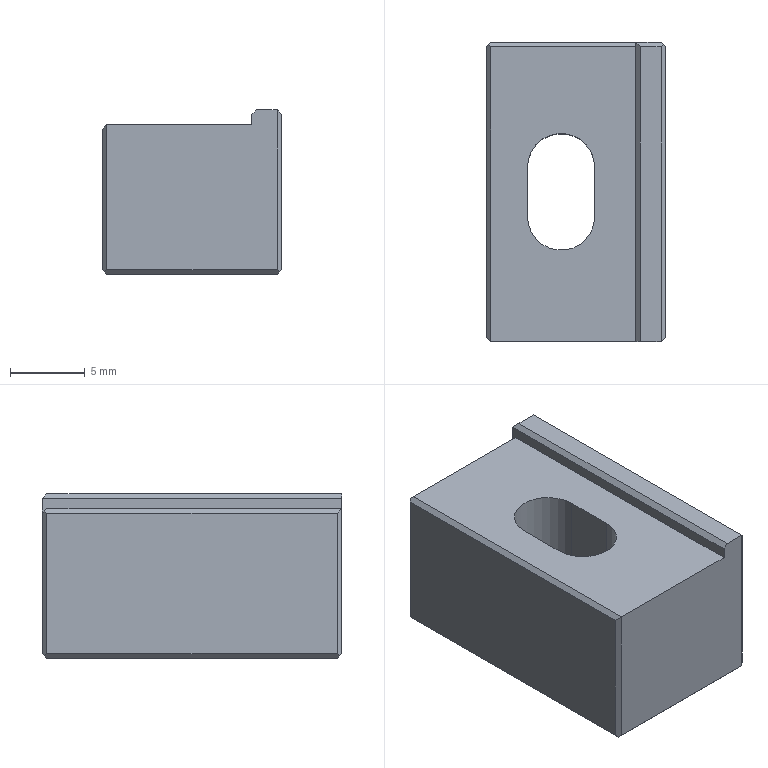Part | NX | 1 solid | 25 faces | box 12 x 20 x 11 mm | volume 2125 mm3 | plane 23 | cylinder 2 | commonest cylinder face diameters 4.5 x2
STEP:
#1=CARTESIAN_POINT('',(2266.8,91.3,-83.));
#2=VERTEX_POINT('',#1);
#3=CARTESIAN_POINT('',(2278.2,91.3,-83.));
#4=VERTEX_POINT('',#3);
#5=CARTESIAN_POINT('',(2272.5,91.3,-83.));
#6=DIRECTION('',(1.,0.,0.));
#7=VECTOR('',#6,1000.);
#8=LINE('',#5,#7);
#9=EDGE_CURVE('',#2,#4,#8,.T.);
#10=ORIENTED_EDGE('',*,*,#9,.F.);
#11=CARTESIAN_POINT('',(2266.8,110.7,-83.));
#12=VERTEX_POINT('',#11);
#13=CARTESIAN_POINT('',(2266.8,101.,-83.));
#14=DIRECTION('',(0.,-1.,0.));
#15=VECTOR('',#14,1000.);
#16=LINE('',#13,#15);
#17=EDGE_CURVE('',#12,#2,#16,.T.);
#18=ORIENTED_EDGE('',*,*,#17,.F.);
#19=CARTESIAN_POINT('',(2278.2,110.7,-83.));
#20=VERTEX_POINT('',#19);
#21=CARTESIAN_POINT('',(2272.5,110.7,-83.));
#22=DIRECTION('',(-1.,0.,0.));
#23=VECTOR('',#22,1000.);
#24=LINE('',#21,#23);
#25=EDGE_CURVE('',#20,#12,#24,.T.);
#26=ORIENTED_EDGE('',*,*,#25,.F.);
#27=CARTESIAN_POINT('',(2278.2,101.,-83.));
#28=DIRECTION('',(0.,-1.,0.));
#29=VECTOR('',#28,1000.);
#30=LINE('',#27,#29);
#31=EDGE_CURVE('',#20,#4,#30,.T.);
#32=ORIENTED_EDGE('',*,*,#31,.T.);
#33=EDGE_LOOP('',(#10,#18,#26,#32));
#34=FACE_BOUND('',#33,.T.);
#35=CARTESIAN_POINT('',(2273.75,99.35,-83.));
#36=VERTEX_POINT('',#35);
#37=CARTESIAN_POINT('',(2269.25,99.35,-83.));
#38=VERTEX_POINT('',#37);
#39=CARTESIAN_POINT('',(2271.5,99.35,-83.));
#40=DIRECTION('',(0.,0.,-1.));
#41=DIRECTION('',(-1.,0.,0.));
#42=AXIS2_PLACEMENT_3D('',#39,#40,#41);
#43=CIRCLE('',#42,2.25);
#44=EDGE_CURVE('',#36,#38,#43,.T.);
#45=ORIENTED_EDGE('',*,*,#44,.F.);
#46=CARTESIAN_POINT('',(2273.75,102.65,-83.));
#47=VERTEX_POINT('',#46);
#48=CARTESIAN_POINT('',(2273.75,45.25,-83.));
#49=DIRECTION('',(0.,1.,0.));
#50=VECTOR('',#49,1000.);
#51=LINE('',#48,#50);
#52=EDGE_CURVE('',#36,#47,#51,.T.);
#53=ORIENTED_EDGE('',*,*,#52,.T.);
#54=CARTESIAN_POINT('',(2269.25,102.65,-83.));
#55=VERTEX_POINT('',#54);
#56=CARTESIAN_POINT('',(2271.5,102.65,-83.));
#57=DIRECTION('',(0.,0.,-1.));
#58=DIRECTION('',(-1.,0.,0.));
#59=AXIS2_PLACEMENT_3D('',#56,#57,#58);
#60=CIRCLE('',#59,2.25);
#61=EDGE_CURVE('',#55,#47,#60,.T.);
#62=ORIENTED_EDGE('',*,*,#61,.F.);
#63=CARTESIAN_POINT('',(2269.25,45.25,-83.));
#64=DIRECTION('',(0.,-1.,0.));
#65=VECTOR('',#64,1000.);
#66=LINE('',#63,#65);
#67=EDGE_CURVE('',#55,#38,#66,.T.);
#68=ORIENTED_EDGE('',*,*,#67,.T.);
#69=EDGE_LOOP('',(#45,#53,#62,#68));
#70=FACE_BOUND('',#69,.T.);
#71=CARTESIAN_POINT('',(2266.5,125.,-83.));
#72=DIRECTION('',(0.,0.,-1.));
#73=DIRECTION('',(0.,-1.,0.));
#74=AXIS2_PLACEMENT_3D('',#71,#72,#73);
#75=PLANE('',#74);
#76=ADVANCED_FACE('',(#34,#70),#75,.T.);
#77=CARTESIAN_POINT('',(2278.2,111.,-72.3));
#78=VERTEX_POINT('',#77);
#79=CARTESIAN_POINT('',(2276.5,111.,-72.3));
#80=VERTEX_POINT('',#79);
#81=CARTESIAN_POINT('',(2277.5,111.,-72.3));
#82=DIRECTION('',(-1.,0.,0.));
#83=VECTOR('',#82,1000.);
#84=LINE('',#81,#83);
#85=EDGE_CURVE('',#78,#80,#84,.T.);
#86=ORIENTED_EDGE('',*,*,#85,.F.);
#87=CARTESIAN_POINT('',(2278.2,111.,-82.7));
#88=VERTEX_POINT('',#87);
#89=CARTESIAN_POINT('',(2278.2,111.,-77.5));
#90=DIRECTION('',(0.,0.,-1.));
#91=VECTOR('',#90,1000.);
#92=LINE('',#89,#91);
#93=EDGE_CURVE('',#78,#88,#92,.T.);
#94=ORIENTED_EDGE('',*,*,#93,.T.);
#95=CARTESIAN_POINT('',(2266.8,111.,-82.7));
#96=VERTEX_POINT('',#95);
#97=CARTESIAN_POINT('',(2272.5,111.,-82.7));
#98=DIRECTION('',(-1.,0.,0.));
#99=VECTOR('',#98,1000.);
#100=LINE('',#97,#99);
#101=EDGE_CURVE('',#88,#96,#100,.T.);
#102=ORIENTED_EDGE('',*,*,#101,.T.);
#103=CARTESIAN_POINT('',(2266.8,111.,-73.3));
#104=VERTEX_POINT('',#103);
#105=CARTESIAN_POINT('',(2266.8,111.,-78.));
#106=DIRECTION('',(0.,0.,-1.));
#107=VECTOR('',#106,1000.);
#108=LINE('',#105,#107);
#109=EDGE_CURVE('',#104,#96,#108,.T.);
#110=ORIENTED_EDGE('',*,*,#109,.F.);
#111=CARTESIAN_POINT('',(2276.5,111.,-73.3));
#112=VERTEX_POINT('',#111);
#113=CARTESIAN_POINT('',(2271.5,111.,-73.3));
#114=DIRECTION('',(-1.,0.,0.));
#115=VECTOR('',#114,1000.);
#116=LINE('',#113,#115);
#117=EDGE_CURVE('',#112,#104,#116,.T.);
#118=ORIENTED_EDGE('',*,*,#117,.F.);
#119=CARTESIAN_POINT('',(2276.5,111.,-12.));
#120=DIRECTION('',(0.,0.,1.));
#121=VECTOR('',#120,1000.);
#122=LINE('',#119,#121);
#123=EDGE_CURVE('',#112,#80,#122,.T.);
#124=ORIENTED_EDGE('',*,*,#123,.T.);
#125=EDGE_LOOP('',(#86,#94,#102,#110,#118,#124));
#126=FACE_BOUND('',#125,.T.);
#127=CARTESIAN_POINT('',(2266.5,111.,-72.));
#128=DIRECTION('',(0.,1.,0.));
#129=DIRECTION('',(1.,0.,0.));
#130=AXIS2_PLACEMENT_3D('',#127,#128,#129);
#131=PLANE('',#130);
#132=ADVANCED_FACE('',(#126),#131,.T.);
#133=CARTESIAN_POINT('',(2276.8,91.,-72.));
#134=VERTEX_POINT('',#133);
#135=CARTESIAN_POINT('',(2276.8,110.7,-72.));
#136=VERTEX_POINT('',#135);
#137=CARTESIAN_POINT('',(2276.8,101.,-72.));
#138=DIRECTION('',(0.,1.,0.));
#139=VECTOR('',#138,1000.);
#140=LINE('',#137,#139);
#141=EDGE_CURVE('',#134,#136,#140,.T.);
#142=ORIENTED_EDGE('',*,*,#141,.F.);
#143=CARTESIAN_POINT('',(2278.2,91.,-72.));
#144=VERTEX_POINT('',#143);
#145=CARTESIAN_POINT('',(2266.5,91.,-72.));
#146=DIRECTION('',(1.,0.,0.));
#147=VECTOR('',#146,1000.);
#148=LINE('',#145,#147);
#149=EDGE_CURVE('',#134,#144,#148,.T.);
#150=ORIENTED_EDGE('',*,*,#149,.T.);
#151=CARTESIAN_POINT('',(2278.2,110.7,-72.));
#152=VERTEX_POINT('',#151);
#153=CARTESIAN_POINT('',(2278.2,101.,-72.));
#154=DIRECTION('',(0.,1.,0.));
#155=VECTOR('',#154,1000.);
#156=LINE('',#153,#155);
#157=EDGE_CURVE('',#144,#152,#156,.T.);
#158=ORIENTED_EDGE('',*,*,#157,.T.);
#159=CARTESIAN_POINT('',(2277.5,110.7,-72.));
#160=DIRECTION('',(-1.,0.,0.));
#161=VECTOR('',#160,1000.);
#162=LINE('',#159,#161);
#163=EDGE_CURVE('',#152,#136,#162,.T.);
#164=ORIENTED_EDGE('',*,*,#163,.T.);
#165=EDGE_LOOP('',(#142,#150,#158,#164));
#166=FACE_BOUND('',#165,.T.);
#167=CARTESIAN_POINT('',(2266.5,91.,-72.));
#168=DIRECTION('',(0.,0.,1.));
#169=DIRECTION('',(1.,0.,0.));
#170=AXIS2_PLACEMENT_3D('',#167,#168,#169);
#171=PLANE('',#170);
#172=ADVANCED_FACE('',(#166),#171,.T.);
#173=CARTESIAN_POINT('',(2276.5,91.,-73.));
#174=VERTEX_POINT('',#173);
#175=CARTESIAN_POINT('',(2276.5,91.,-72.3));
#176=VERTEX_POINT('',#175);
#177=CARTESIAN_POINT('',(2276.5,91.,-12.));
#178=DIRECTION('',(0.,0.,1.));
#179=VECTOR('',#178,1000.);
#180=LINE('',#177,#179);
#181=EDGE_CURVE('',#174,#176,#180,.T.);
#182=ORIENTED_EDGE('',*,*,#181,.F.);
#183=CARTESIAN_POINT('',(2266.8,91.,-73.));
#184=VERTEX_POINT('',#183);
#185=CARTESIAN_POINT('',(2266.5,91.,-73.));
#186=DIRECTION('',(-1.,0.,0.));
#187=VECTOR('',#186,1000.);
#188=LINE('',#185,#187);
#189=EDGE_CURVE('',#174,#184,#188,.T.);
#190=ORIENTED_EDGE('',*,*,#189,.T.);
#191=CARTESIAN_POINT('',(2266.8,91.,-82.7));
#192=VERTEX_POINT('',#191);
#193=CARTESIAN_POINT('',(2266.8,91.,-78.));
#194=DIRECTION('',(0.,0.,1.));
#195=VECTOR('',#194,1000.);
#196=LINE('',#193,#195);
#197=EDGE_CURVE('',#192,#184,#196,.T.);
#198=ORIENTED_EDGE('',*,*,#197,.F.);
#199=CARTESIAN_POINT('',(2278.2,91.,-82.7));
#200=VERTEX_POINT('',#199);
#201=CARTESIAN_POINT('',(2272.5,91.,-82.7));
#202=DIRECTION('',(1.,0.,0.));
#203=VECTOR('',#202,1000.);
#204=LINE('',#201,#203);
#205=EDGE_CURVE('',#192,#200,#204,.T.);
#206=ORIENTED_EDGE('',*,*,#205,.T.);
#207=CARTESIAN_POINT('',(2278.2,91.,-77.5));
#208=DIRECTION('',(0.,0.,1.));
#209=VECTOR('',#208,1000.);
#210=LINE('',#207,#209);
#211=EDGE_CURVE('',#200,#144,#210,.T.);
#212=ORIENTED_EDGE('',*,*,#211,.T.);
#213=ORIENTED_EDGE('',*,*,#149,.F.);
#214=CARTESIAN_POINT('',(2266.5,91.,-82.3));
#215=DIRECTION('',(-0.7071,0.,-0.7071));
#216=VECTOR('',#215,1000.);
#217=LINE('',#214,#216);
#218=EDGE_CURVE('',#134,#176,#217,.T.);
#219=ORIENTED_EDGE('',*,*,#218,.T.);
#220=EDGE_LOOP('',(#182,#190,#198,#206,#212,#213,#219));
#221=FACE_BOUND('',#220,.T.);
#222=CARTESIAN_POINT('',(2266.5,91.,-81.));
#223=DIRECTION('',(0.,-1.,0.));
#224=DIRECTION('',(0.,0.,-1.));
#225=AXIS2_PLACEMENT_3D('',#222,#223,#224);
#226=PLANE('',#225);
#227=ADVANCED_FACE('',(#221),#226,.T.);
#228=CARTESIAN_POINT('',(2266.8,110.7,-73.));
#229=VERTEX_POINT('',#228);
#230=CARTESIAN_POINT('',(2266.8,101.,-73.));
#231=DIRECTION('',(0.,1.,0.));
#232=VECTOR('',#231,1000.);
#233=LINE('',#230,#232);
#234=EDGE_CURVE('',#184,#229,#233,.T.);
#235=ORIENTED_EDGE('',*,*,#234,.F.);
#236=ORIENTED_EDGE('',*,*,#189,.F.);
#237=CARTESIAN_POINT('',(2276.5,110.7,-73.));
#238=VERTEX_POINT('',#237);
#239=CARTESIAN_POINT('',(2276.5,45.25,-73.));
#240=DIRECTION('',(0.,-1.,0.));
#241=VECTOR('',#240,1000.);
#242=LINE('',#239,#241);
#243=EDGE_CURVE('',#238,#174,#242,.T.);
#244=ORIENTED_EDGE('',*,*,#243,.F.);
#245=CARTESIAN_POINT('',(2271.5,110.7,-73.));
#246=DIRECTION('',(-1.,0.,0.));
#247=VECTOR('',#246,1000.);
#248=LINE('',#245,#247);
#249=EDGE_CURVE('',#238,#229,#248,.T.);
#250=ORIENTED_EDGE('',*,*,#249,.T.);
#251=EDGE_LOOP('',(#235,#236,#244,#250));
#252=FACE_BOUND('',#251,.T.);
#253=CARTESIAN_POINT('',(2273.75,99.35,-73.));
#254=VERTEX_POINT('',#253);
#255=CARTESIAN_POINT('',(2269.25,99.35,-73.));
#256=VERTEX_POINT('',#255);
#257=CARTESIAN_POINT('',(2271.5,99.35,-73.));
#258=DIRECTION('',(0.,0.,-1.));
#259=DIRECTION('',(-1.,0.,0.));
#260=AXIS2_PLACEMENT_3D('',#257,#258,#259);
#261=CIRCLE('',#260,2.25);
#262=EDGE_CURVE('',#254,#256,#261,.T.);
#263=ORIENTED_EDGE('',*,*,#262,.T.);
#264=CARTESIAN_POINT('',(2269.25,102.65,-73.));
#265=VERTEX_POINT('',#264);
#266=CARTESIAN_POINT('',(2269.25,45.25,-73.));
#267=DIRECTION('',(0.,1.,0.));
#268=VECTOR('',#267,1000.);
#269=LINE('',#266,#268);
#270=EDGE_CURVE('',#256,#265,#269,.T.);
#271=ORIENTED_EDGE('',*,*,#270,.T.);
#272=CARTESIAN_POINT('',(2273.75,102.65,-73.));
#273=VERTEX_POINT('',#272);
#274=CARTESIAN_POINT('',(2271.5,102.65,-73.));
#275=DIRECTION('',(0.,0.,-1.));
#276=DIRECTION('',(-1.,0.,0.));
#277=AXIS2_PLACEMENT_3D('',#274,#275,#276);
#278=CIRCLE('',#277,2.25);
#279=EDGE_CURVE('',#265,#273,#278,.T.);
#280=ORIENTED_EDGE('',*,*,#279,.T.);
#281=CARTESIAN_POINT('',(2273.75,45.25,-73.));
#282=DIRECTION('',(0.,-1.,0.));
#283=VECTOR('',#282,1000.);
#284=LINE('',#281,#283);
#285=EDGE_CURVE('',#273,#254,#284,.T.);
#286=ORIENTED_EDGE('',*,*,#285,.T.);
#287=EDGE_LOOP('',(#263,#271,#280,#286));
#288=FACE_BOUND('',#287,.T.);
#289=CARTESIAN_POINT('',(2275.402,98.391,-73.));
#290=DIRECTION('',(0.,0.,1.));
#291=DIRECTION('',(1.,0.,0.));
#292=AXIS2_PLACEMENT_3D('',#289,#290,#291);
#293=PLANE('',#292);
#294=ADVANCED_FACE('',(#252,#288),#293,.T.);
#295=ORIENTED_EDGE('',*,*,#123,.F.);
#296=CARTESIAN_POINT('',(2276.5,49.7,-12.));
#297=DIRECTION('',(0.,0.7071,-0.7071));
#298=VECTOR('',#297,1000.);
#299=LINE('',#296,#298);
#300=EDGE_CURVE('',#238,#112,#299,.T.);
#301=ORIENTED_EDGE('',*,*,#300,.F.);
#302=ORIENTED_EDGE('',*,*,#243,.T.);
#303=ORIENTED_EDGE('',*,*,#181,.T.);
#304=CARTESIAN_POINT('',(2276.5,101.,-72.3));
#305=DIRECTION('',(0.,1.,0.));
#306=VECTOR('',#305,1000.);
#307=LINE('',#304,#306);
#308=EDGE_CURVE('',#176,#80,#307,.T.);
#309=ORIENTED_EDGE('',*,*,#308,.T.);
#310=EDGE_LOOP('',(#295,#301,#302,#303,#309));
#311=FACE_BOUND('',#310,.T.);
#312=CARTESIAN_POINT('',(2276.5,91.,-72.));
#313=DIRECTION('',(1.,0.,0.));
#314=DIRECTION('',(0.,1.,0.));
#315=AXIS2_PLACEMENT_3D('',#312,#313,#314);
#316=PLANE('',#315);
#317=ADVANCED_FACE('',(#311),#316,.F.);
#318=ORIENTED_EDGE('',*,*,#262,.F.);
#319=CARTESIAN_POINT('',(2273.75,99.35,-71.1));
#320=DIRECTION('',(0.,0.,-1.));
#321=VECTOR('',#320,1000.);
#322=LINE('',#319,#321);
#323=EDGE_CURVE('',#254,#36,#322,.T.);
#324=ORIENTED_EDGE('',*,*,#323,.T.);
#325=ORIENTED_EDGE('',*,*,#44,.T.);
#326=CARTESIAN_POINT('',(2269.25,99.35,-71.1));
#327=DIRECTION('',(0.,0.,-1.));
#328=VECTOR('',#327,1000.);
#329=LINE('',#326,#328);
#330=EDGE_CURVE('',#256,#38,#329,.T.);
#331=ORIENTED_EDGE('',*,*,#330,.F.);
#332=EDGE_LOOP('',(#318,#324,#325,#331));
#333=FACE_BOUND('',#332,.T.);
#334=CARTESIAN_POINT('',(2271.5,99.35,-71.1));
#335=DIRECTION('',(0.,0.,-1.));
#336=DIRECTION('',(-1.,0.,0.));
#337=AXIS2_PLACEMENT_3D('',#334,#335,#336);
#338=CYLINDRICAL_SURFACE('',#337,2.25);
#339=ADVANCED_FACE('',(#333),#338,.F.);
#340=ORIENTED_EDGE('',*,*,#285,.F.);
#341=CARTESIAN_POINT('',(2273.75,102.65,-71.1));
#342=DIRECTION('',(0.,0.,-1.));
#343=VECTOR('',#342,1000.);
#344=LINE('',#341,#343);
#345=EDGE_CURVE('',#273,#47,#344,.T.);
#346=ORIENTED_EDGE('',*,*,#345,.T.);
#347=ORIENTED_EDGE('',*,*,#52,.F.);
#348=ORIENTED_EDGE('',*,*,#323,.F.);
#349=EDGE_LOOP('',(#340,#346,#347,#348));
#350=FACE_BOUND('',#349,.T.);
#351=CARTESIAN_POINT('',(2273.75,99.35,-71.1));
#352=DIRECTION('',(1.,0.,0.));
#353=DIRECTION('',(0.,1.,0.));
#354=AXIS2_PLACEMENT_3D('',#351,#352,#353);
#355=PLANE('',#354);
#356=ADVANCED_FACE('',(#350),#355,.F.);
#357=ORIENTED_EDGE('',*,*,#279,.F.);
#358=CARTESIAN_POINT('',(2269.25,102.65,-71.1));
#359=DIRECTION('',(0.,0.,-1.));
#360=VECTOR('',#359,1000.);
#361=LINE('',#358,#360);
#362=EDGE_CURVE('',#265,#55,#361,.T.);
#363=ORIENTED_EDGE('',*,*,#362,.T.);
#364=ORIENTED_EDGE('',*,*,#61,.T.);
#365=ORIENTED_EDGE('',*,*,#345,.F.);
#366=EDGE_LOOP('',(#357,#363,#364,#365));
#367=FACE_BOUND('',#366,.T.);
#368=CARTESIAN_POINT('',(2271.5,102.65,-71.1));
#369=DIRECTION('',(0.,0.,-1.));
#370=DIRECTION('',(-1.,0.,0.));
#371=AXIS2_PLACEMENT_3D('',#368,#369,#370);
#372=CYLINDRICAL_SURFACE('',#371,2.25);
#373=ADVANCED_FACE('',(#367),#372,.F.);
#374=ORIENTED_EDGE('',*,*,#270,.F.);
#375=ORIENTED_EDGE('',*,*,#330,.T.);
#376=ORIENTED_EDGE('',*,*,#67,.F.);
#377=ORIENTED_EDGE('',*,*,#362,.F.);
#378=EDGE_LOOP('',(#374,#375,#376,#377));
#379=FACE_BOUND('',#378,.T.);
#380=CARTESIAN_POINT('',(2269.25,102.65,-71.1));
#381=DIRECTION('',(-1.,0.,0.));
#382=DIRECTION('',(0.,0.,1.));
#383=AXIS2_PLACEMENT_3D('',#380,#381,#382);
#384=PLANE('',#383);
#385=ADVANCED_FACE('',(#379),#384,.F.);
#386=ORIENTED_EDGE('',*,*,#25,.T.);
#387=CARTESIAN_POINT('',(2266.65,110.85,-82.85));
#388=VERTEX_POINT('',#387);
#389=CARTESIAN_POINT('',(2266.5,111.,-82.7));
#390=DIRECTION('',(0.5774,-0.5774,-0.5774));
#391=VECTOR('',#390,1000.);
#392=LINE('',#389,#391);
#393=EDGE_CURVE('',#388,#12,#392,.T.);
#394=ORIENTED_EDGE('',*,*,#393,.F.);
#395=CARTESIAN_POINT('',(2266.5,110.7,-83.));
#396=DIRECTION('',(-0.5774,-0.5774,-0.5774));
#397=VECTOR('',#396,1000.);
#398=LINE('',#395,#397);
#399=EDGE_CURVE('',#96,#388,#398,.T.);
#400=ORIENTED_EDGE('',*,*,#399,.F.);
#401=ORIENTED_EDGE('',*,*,#101,.F.);
#402=CARTESIAN_POINT('',(2278.35,110.85,-82.85));
#403=VERTEX_POINT('',#402);
#404=CARTESIAN_POINT('',(2266.5,122.7,-71.));
#405=DIRECTION('',(0.5774,-0.5774,-0.5774));
#406=VECTOR('',#405,1000.);
#407=LINE('',#404,#406);
#408=EDGE_CURVE('',#88,#403,#407,.T.);
#409=ORIENTED_EDGE('',*,*,#408,.T.);
#410=CARTESIAN_POINT('',(2266.5,99.,-94.7));
#411=DIRECTION('',(-0.5774,-0.5774,-0.5774));
#412=VECTOR('',#411,1000.);
#413=LINE('',#410,#412);
#414=EDGE_CURVE('',#403,#20,#413,.T.);
#415=ORIENTED_EDGE('',*,*,#414,.T.);
#416=EDGE_LOOP('',(#386,#394,#400,#401,#409,#415));
#417=FACE_BOUND('',#416,.T.);
#418=CARTESIAN_POINT('',(2272.5,110.85,-82.85));
#419=DIRECTION('',(0.,-0.7071,0.7071));
#420=DIRECTION('',(-1.,0.,0.));
#421=AXIS2_PLACEMENT_3D('',#418,#419,#420);
#422=PLANE('',#421);
#423=ADVANCED_FACE('',(#417),#422,.F.);
#424=ORIENTED_EDGE('',*,*,#249,.F.);
#425=ORIENTED_EDGE('',*,*,#300,.T.);
#426=ORIENTED_EDGE('',*,*,#117,.T.);
#427=CARTESIAN_POINT('',(2266.65,110.85,-73.15));
#428=VERTEX_POINT('',#427);
#429=CARTESIAN_POINT('',(2266.5,110.7,-73.));
#430=DIRECTION('',(0.5774,0.5774,-0.5774));
#431=VECTOR('',#430,1000.);
#432=LINE('',#429,#431);
#433=EDGE_CURVE('',#428,#104,#432,.T.);
#434=ORIENTED_EDGE('',*,*,#433,.F.);
#435=CARTESIAN_POINT('',(2266.5,111.,-73.3));
#436=DIRECTION('',(-0.5774,0.5774,-0.5774));
#437=VECTOR('',#436,1000.);
#438=LINE('',#435,#437);
#439=EDGE_CURVE('',#229,#428,#438,.T.);
#440=ORIENTED_EDGE('',*,*,#439,.F.);
#441=EDGE_LOOP('',(#424,#425,#426,#434,#440));
#442=FACE_BOUND('',#441,.T.);
#443=CARTESIAN_POINT('',(2271.5,110.85,-73.15));
#444=DIRECTION('',(0.,0.7071,0.7071));
#445=DIRECTION('',(1.,0.,0.));
#446=AXIS2_PLACEMENT_3D('',#443,#444,#445);
#447=PLANE('',#446);
#448=ADVANCED_FACE('',(#442),#447,.T.);
#449=ORIENTED_EDGE('',*,*,#85,.T.);
#450=CARTESIAN_POINT('',(2266.5,121.,-82.3));
#451=DIRECTION('',(0.5774,-0.5774,0.5774));
#452=VECTOR('',#451,1000.);
#453=LINE('',#450,#452);
#454=EDGE_CURVE('',#80,#136,#453,.T.);
#455=ORIENTED_EDGE('',*,*,#454,.T.);
#456=ORIENTED_EDGE('',*,*,#163,.F.);
#457=CARTESIAN_POINT('',(2278.35,110.85,-72.15));
#458=VERTEX_POINT('',#457);
#459=CARTESIAN_POINT('',(2266.5,99.,-60.3));
#460=DIRECTION('',(0.5774,0.5774,-0.5774));
#461=VECTOR('',#460,1000.);
#462=LINE('',#459,#461);
#463=EDGE_CURVE('',#152,#458,#462,.T.);
#464=ORIENTED_EDGE('',*,*,#463,.T.);
#465=CARTESIAN_POINT('',(2266.5,122.7,-84.));
#466=DIRECTION('',(-0.5774,0.5774,-0.5774));
#467=VECTOR('',#466,1000.);
#468=LINE('',#465,#467);
#469=EDGE_CURVE('',#458,#78,#468,.T.);
#470=ORIENTED_EDGE('',*,*,#469,.T.);
#471=EDGE_LOOP('',(#449,#455,#456,#464,#470));
#472=FACE_BOUND('',#471,.T.);
#473=CARTESIAN_POINT('',(2277.5,110.85,-72.15));
#474=DIRECTION('',(0.,-0.7071,-0.7071));
#475=DIRECTION('',(0.,-0.7071,0.7071));
#476=AXIS2_PLACEMENT_3D('',#473,#474,#475);
#477=PLANE('',#476);
#478=ADVANCED_FACE('',(#472),#477,.F.);
#479=ORIENTED_EDGE('',*,*,#141,.T.);
#480=ORIENTED_EDGE('',*,*,#454,.F.);
#481=ORIENTED_EDGE('',*,*,#308,.F.);
#482=ORIENTED_EDGE('',*,*,#218,.F.);
#483=EDGE_LOOP('',(#479,#480,#481,#482));
#484=FACE_BOUND('',#483,.T.);
#485=CARTESIAN_POINT('',(2276.65,101.,-72.15));
#486=DIRECTION('',(0.7071,0.,-0.7071));
#487=DIRECTION('',(0.,-1.,0.));
#488=AXIS2_PLACEMENT_3D('',#485,#486,#487);
#489=PLANE('',#488);
#490=ADVANCED_FACE('',(#484),#489,.F.);
#491=ORIENTED_EDGE('',*,*,#234,.T.);
#492=ORIENTED_EDGE('',*,*,#439,.T.);
#493=CARTESIAN_POINT('',(2266.5,110.7,-73.3));
#494=VERTEX_POINT('',#493);
#495=CARTESIAN_POINT('',(2266.5,110.7,-73.3));
#496=DIRECTION('',(-0.5774,-0.5774,-0.5774));
#497=VECTOR('',#496,1000.);
#498=LINE('',#495,#497);
#499=EDGE_CURVE('',#428,#494,#498,.T.);
#500=ORIENTED_EDGE('',*,*,#499,.T.);
#501=CARTESIAN_POINT('',(2266.5,91.3,-73.3));
#502=VERTEX_POINT('',#501);
#503=CARTESIAN_POINT('',(2266.5,101.,-73.3));
#504=DIRECTION('',(0.,1.,0.));
#505=VECTOR('',#504,1000.);
#506=LINE('',#503,#505);
#507=EDGE_CURVE('',#502,#494,#506,.T.);
#508=ORIENTED_EDGE('',*,*,#507,.F.);
#509=CARTESIAN_POINT('',(2266.5,91.3,-73.3));
#510=DIRECTION('',(-0.5774,0.5774,-0.5774));
#511=VECTOR('',#510,1000.);
#512=LINE('',#509,#511);
#513=EDGE_CURVE('',#184,#502,#512,.T.);
#514=ORIENTED_EDGE('',*,*,#513,.F.);
#515=EDGE_LOOP('',(#491,#492,#500,#508,#514));
#516=FACE_BOUND('',#515,.T.);
#517=CARTESIAN_POINT('',(2266.65,101.,-73.15));
#518=DIRECTION('',(0.7071,0.,-0.7071));
#519=DIRECTION('',(0.,-1.,0.));
#520=AXIS2_PLACEMENT_3D('',#517,#518,#519);
#521=PLANE('',#520);
#522=ADVANCED_FACE('',(#516),#521,.F.);
#523=ORIENTED_EDGE('',*,*,#9,.T.);
#524=CARTESIAN_POINT('',(2278.35,91.15,-82.85));
#525=VERTEX_POINT('',#524);
#526=CARTESIAN_POINT('',(2266.5,103.,-94.7));
#527=DIRECTION('',(0.5774,-0.5774,0.5774));
#528=VECTOR('',#527,1000.);
#529=LINE('',#526,#528);
#530=EDGE_CURVE('',#4,#525,#529,.T.);
#531=ORIENTED_EDGE('',*,*,#530,.T.);
#532=CARTESIAN_POINT('',(2266.5,79.3,-71.));
#533=DIRECTION('',(0.5774,0.5774,-0.5774));
#534=VECTOR('',#533,1000.);
#535=LINE('',#532,#534);
#536=EDGE_CURVE('',#200,#525,#535,.T.);
#537=ORIENTED_EDGE('',*,*,#536,.F.);
#538=ORIENTED_EDGE('',*,*,#205,.F.);
#539=CARTESIAN_POINT('',(2266.65,91.15,-82.85));
#540=VERTEX_POINT('',#539);
#541=CARTESIAN_POINT('',(2266.5,91.3,-83.));
#542=DIRECTION('',(-0.5774,0.5774,-0.5774));
#543=VECTOR('',#542,1000.);
#544=LINE('',#541,#543);
#545=EDGE_CURVE('',#192,#540,#544,.T.);
#546=ORIENTED_EDGE('',*,*,#545,.T.);
#547=CARTESIAN_POINT('',(2266.5,91.,-82.7));
#548=DIRECTION('',(0.5774,0.5774,-0.5774));
#549=VECTOR('',#548,1000.);
#550=LINE('',#547,#549);
#551=EDGE_CURVE('',#540,#2,#550,.T.);
#552=ORIENTED_EDGE('',*,*,#551,.T.);
#553=EDGE_LOOP('',(#523,#531,#537,#538,#546,#552));
#554=FACE_BOUND('',#553,.T.);
#555=CARTESIAN_POINT('',(2272.5,91.15,-82.85));
#556=DIRECTION('',(0.,0.7071,0.7071));
#557=DIRECTION('',(1.,0.,0.));
#558=AXIS2_PLACEMENT_3D('',#555,#556,#557);
#559=PLANE('',#558);
#560=ADVANCED_FACE('',(#554),#559,.F.);
#561=CARTESIAN_POINT('',(2278.5,110.7,-82.7));
#562=VERTEX_POINT('',#561);
#563=CARTESIAN_POINT('',(2278.5,91.3,-82.7));
#564=VERTEX_POINT('',#563);
#565=CARTESIAN_POINT('',(2278.5,101.,-82.7));
#566=DIRECTION('',(0.,-1.,0.));
#567=VECTOR('',#566,1000.);
#568=LINE('',#565,#567);
#569=EDGE_CURVE('',#562,#564,#568,.T.);
#570=ORIENTED_EDGE('',*,*,#569,.F.);
#571=CARTESIAN_POINT('',(2278.5,110.7,-72.3));
#572=VERTEX_POINT('',#571);
#573=CARTESIAN_POINT('',(2278.5,110.7,-77.5));
#574=DIRECTION('',(0.,0.,-1.));
#575=VECTOR('',#574,1000.);
#576=LINE('',#573,#575);
#577=EDGE_CURVE('',#572,#562,#576,.T.);
#578=ORIENTED_EDGE('',*,*,#577,.F.);
#579=CARTESIAN_POINT('',(2278.5,91.3,-72.3));
#580=VERTEX_POINT('',#579);
#581=CARTESIAN_POINT('',(2278.5,101.,-72.3));
#582=DIRECTION('',(0.,1.,0.));
#583=VECTOR('',#582,1000.);
#584=LINE('',#581,#583);
#585=EDGE_CURVE('',#580,#572,#584,.T.);
#586=ORIENTED_EDGE('',*,*,#585,.F.);
#587=CARTESIAN_POINT('',(2278.5,91.3,-77.5));
#588=DIRECTION('',(0.,0.,1.));
#589=VECTOR('',#588,1000.);
#590=LINE('',#587,#589);
#591=EDGE_CURVE('',#564,#580,#590,.T.);
#592=ORIENTED_EDGE('',*,*,#591,.F.);
#593=EDGE_LOOP('',(#570,#578,#586,#592));
#594=FACE_BOUND('',#593,.T.);
#595=CARTESIAN_POINT('',(2278.5,45.25,-12.));
#596=DIRECTION('',(-1.,0.,0.));
#597=DIRECTION('',(0.,0.,1.));
#598=AXIS2_PLACEMENT_3D('',#595,#596,#597);
#599=PLANE('',#598);
#600=ADVANCED_FACE('',(#594),#599,.F.);
#601=ORIENTED_EDGE('',*,*,#577,.T.);
#602=CARTESIAN_POINT('',(2266.5,122.7,-94.7));
#603=DIRECTION('',(-0.5774,0.5774,-0.5774));
#604=VECTOR('',#603,1000.);
#605=LINE('',#602,#604);
#606=EDGE_CURVE('',#562,#403,#605,.T.);
#607=ORIENTED_EDGE('',*,*,#606,.T.);
#608=ORIENTED_EDGE('',*,*,#408,.F.);
#609=ORIENTED_EDGE('',*,*,#93,.F.);
#610=ORIENTED_EDGE('',*,*,#469,.F.);
#611=CARTESIAN_POINT('',(2266.5,122.7,-60.3));
#612=DIRECTION('',(0.5774,-0.5774,-0.5774));
#613=VECTOR('',#612,1000.);
#614=LINE('',#611,#613);
#615=EDGE_CURVE('',#458,#572,#614,.T.);
#616=ORIENTED_EDGE('',*,*,#615,.T.);
#617=EDGE_LOOP('',(#601,#607,#608,#609,#610,#616));
#618=FACE_BOUND('',#617,.T.);
#619=CARTESIAN_POINT('',(2278.35,110.85,-77.5));
#620=DIRECTION('',(-0.7071,-0.7071,0.));
#621=DIRECTION('',(-0.7071,0.7071,0.));
#622=AXIS2_PLACEMENT_3D('',#619,#620,#621);
#623=PLANE('',#622);
#624=ADVANCED_FACE('',(#618),#623,.F.);
#625=ORIENTED_EDGE('',*,*,#591,.T.);
#626=CARTESIAN_POINT('',(2266.5,79.3,-60.3));
#627=DIRECTION('',(-0.5774,-0.5774,0.5774));
#628=VECTOR('',#627,1000.);
#629=LINE('',#626,#628);
#630=EDGE_CURVE('',#580,#144,#629,.T.);
#631=ORIENTED_EDGE('',*,*,#630,.T.);
#632=ORIENTED_EDGE('',*,*,#211,.F.);
#633=ORIENTED_EDGE('',*,*,#536,.T.);
#634=CARTESIAN_POINT('',(2266.5,79.3,-94.7));
#635=DIRECTION('',(0.5774,0.5774,0.5774));
#636=VECTOR('',#635,1000.);
#637=LINE('',#634,#636);
#638=EDGE_CURVE('',#525,#564,#637,.T.);
#639=ORIENTED_EDGE('',*,*,#638,.T.);
#640=EDGE_LOOP('',(#625,#631,#632,#633,#639));
#641=FACE_BOUND('',#640,.T.);
#642=CARTESIAN_POINT('',(2278.35,91.15,-77.5));
#643=DIRECTION('',(-0.7071,0.7071,0.));
#644=DIRECTION('',(0.,0.,1.));
#645=AXIS2_PLACEMENT_3D('',#642,#643,#644);
#646=PLANE('',#645);
#647=ADVANCED_FACE('',(#641),#646,.F.);
#648=ORIENTED_EDGE('',*,*,#585,.T.);
#649=ORIENTED_EDGE('',*,*,#615,.F.);
#650=ORIENTED_EDGE('',*,*,#463,.F.);
#651=ORIENTED_EDGE('',*,*,#157,.F.);
#652=ORIENTED_EDGE('',*,*,#630,.F.);
#653=EDGE_LOOP('',(#648,#649,#650,#651,#652));
#654=FACE_BOUND('',#653,.T.);
#655=CARTESIAN_POINT('',(2278.35,101.,-72.15));
#656=DIRECTION('',(-0.7071,0.,-0.7071));
#657=DIRECTION('',(-0.7071,0.,0.7071));
#658=AXIS2_PLACEMENT_3D('',#655,#656,#657);
#659=PLANE('',#658);
#660=ADVANCED_FACE('',(#654),#659,.F.);
#661=ORIENTED_EDGE('',*,*,#569,.T.);
#662=ORIENTED_EDGE('',*,*,#638,.F.);
#663=ORIENTED_EDGE('',*,*,#530,.F.);
#664=ORIENTED_EDGE('',*,*,#31,.F.);
#665=ORIENTED_EDGE('',*,*,#414,.F.);
#666=ORIENTED_EDGE('',*,*,#606,.F.);
#667=EDGE_LOOP('',(#661,#662,#663,#664,#665,#666));
#668=FACE_BOUND('',#667,.T.);
#669=CARTESIAN_POINT('',(2278.35,101.,-82.85));
#670=DIRECTION('',(-0.7071,0.,0.7071));
#671=DIRECTION('',(0.,1.,0.));
#672=AXIS2_PLACEMENT_3D('',#669,#670,#671);
#673=PLANE('',#672);
#674=ADVANCED_FACE('',(#668),#673,.F.);
#675=CARTESIAN_POINT('',(2266.5,91.3,-82.7));
#676=VERTEX_POINT('',#675);
#677=CARTESIAN_POINT('',(2266.5,91.3,-78.));
#678=DIRECTION('',(0.,0.,1.));
#679=VECTOR('',#678,1000.);
#680=LINE('',#677,#679);
#681=EDGE_CURVE('',#676,#502,#680,.T.);
#682=ORIENTED_EDGE('',*,*,#681,.T.);
#683=ORIENTED_EDGE('',*,*,#507,.T.);
#684=CARTESIAN_POINT('',(2266.5,110.7,-82.7));
#685=VERTEX_POINT('',#684);
#686=CARTESIAN_POINT('',(2266.5,110.7,-78.));
#687=DIRECTION('',(0.,0.,-1.));
#688=VECTOR('',#687,1000.);
#689=LINE('',#686,#688);
#690=EDGE_CURVE('',#494,#685,#689,.T.);
#691=ORIENTED_EDGE('',*,*,#690,.T.);
#692=CARTESIAN_POINT('',(2266.5,101.,-82.7));
#693=DIRECTION('',(0.,-1.,0.));
#694=VECTOR('',#693,1000.);
#695=LINE('',#692,#694);
#696=EDGE_CURVE('',#685,#676,#695,.T.);
#697=ORIENTED_EDGE('',*,*,#696,.T.);
#698=EDGE_LOOP('',(#682,#683,#691,#697));
#699=FACE_BOUND('',#698,.T.);
#700=CARTESIAN_POINT('',(2266.5,45.25,-12.));
#701=DIRECTION('',(-1.,0.,0.));
#702=DIRECTION('',(0.,0.,1.));
#703=AXIS2_PLACEMENT_3D('',#700,#701,#702);
#704=PLANE('',#703);
#705=ADVANCED_FACE('',(#699),#704,.T.);
#706=ORIENTED_EDGE('',*,*,#696,.F.);
#707=CARTESIAN_POINT('',(2266.5,110.7,-82.7));
#708=DIRECTION('',(0.5774,0.5774,-0.5774));
#709=VECTOR('',#708,1000.);
#710=LINE('',#707,#709);
#711=EDGE_CURVE('',#685,#388,#710,.T.);
#712=ORIENTED_EDGE('',*,*,#711,.T.);
#713=ORIENTED_EDGE('',*,*,#393,.T.);
#714=ORIENTED_EDGE('',*,*,#17,.T.);
#715=ORIENTED_EDGE('',*,*,#551,.F.);
#716=CARTESIAN_POINT('',(2266.5,91.3,-82.7));
#717=DIRECTION('',(-0.5774,0.5774,0.5774));
#718=VECTOR('',#717,1000.);
#719=LINE('',#716,#718);
#720=EDGE_CURVE('',#540,#676,#719,.T.);
#721=ORIENTED_EDGE('',*,*,#720,.T.);
#722=EDGE_LOOP('',(#706,#712,#713,#714,#715,#721));
#723=FACE_BOUND('',#722,.T.);
#724=CARTESIAN_POINT('',(2266.65,101.,-82.85));
#725=DIRECTION('',(-0.7071,0.,-0.7071));
#726=DIRECTION('',(-0.7071,0.,0.7071));
#727=AXIS2_PLACEMENT_3D('',#724,#725,#726);
#728=PLANE('',#727);
#729=ADVANCED_FACE('',(#723),#728,.T.);
#730=ORIENTED_EDGE('',*,*,#690,.F.);
#731=ORIENTED_EDGE('',*,*,#499,.F.);
#732=ORIENTED_EDGE('',*,*,#433,.T.);
#733=ORIENTED_EDGE('',*,*,#109,.T.);
#734=ORIENTED_EDGE('',*,*,#399,.T.);
#735=ORIENTED_EDGE('',*,*,#711,.F.);
#736=EDGE_LOOP('',(#730,#731,#732,#733,#734,#735));
#737=FACE_BOUND('',#736,.T.);
#738=CARTESIAN_POINT('',(2266.65,110.85,-78.));
#739=DIRECTION('',(-0.7071,0.7071,0.));
#740=DIRECTION('',(0.,0.,1.));
#741=AXIS2_PLACEMENT_3D('',#738,#739,#740);
#742=PLANE('',#741);
#743=ADVANCED_FACE('',(#737),#742,.T.);
#744=ORIENTED_EDGE('',*,*,#681,.F.);
#745=ORIENTED_EDGE('',*,*,#720,.F.);
#746=ORIENTED_EDGE('',*,*,#545,.F.);
#747=ORIENTED_EDGE('',*,*,#197,.T.);
#748=ORIENTED_EDGE('',*,*,#513,.T.);
#749=EDGE_LOOP('',(#744,#745,#746,#747,#748));
#750=FACE_BOUND('',#749,.T.);
#751=CARTESIAN_POINT('',(2266.65,91.15,-78.));
#752=DIRECTION('',(-0.7071,-0.7071,0.));
#753=DIRECTION('',(-0.7071,0.7071,0.));
#754=AXIS2_PLACEMENT_3D('',#751,#752,#753);
#755=PLANE('',#754);
#756=ADVANCED_FACE('',(#750),#755,.T.);
#757=CLOSED_SHELL('',(#76,#132,#172,#227,#294,#317,#339,#356,#373,#385,#423,#448,#478,#490,#522,#560,#600,#624,#647,#660,#674,#705,#729,#743,#756));
#758=MANIFOLD_SOLID_BREP('',#757);
#759=(LENGTH_UNIT()NAMED_UNIT(*)SI_UNIT(.MILLI.,.METRE.));
#760=UNCERTAINTY_MEASURE_WITH_UNIT(LENGTH_MEASURE(0.00001),#759,'','');
#761=(NAMED_UNIT(*)PLANE_ANGLE_UNIT()SI_UNIT($,.RADIAN.));
#762=(NAMED_UNIT(*)SI_UNIT($,.STERADIAN.)SOLID_ANGLE_UNIT());
#763=(GEOMETRIC_REPRESENTATION_CONTEXT(3)GLOBAL_UNCERTAINTY_ASSIGNED_CONTEXT((#760))GLOBAL_UNIT_ASSIGNED_CONTEXT((#759,#761,#762))REPRESENTATION_CONTEXT('',''));
#764=ADVANCED_BREP_SHAPE_REPRESENTATION('',(#758),#763);